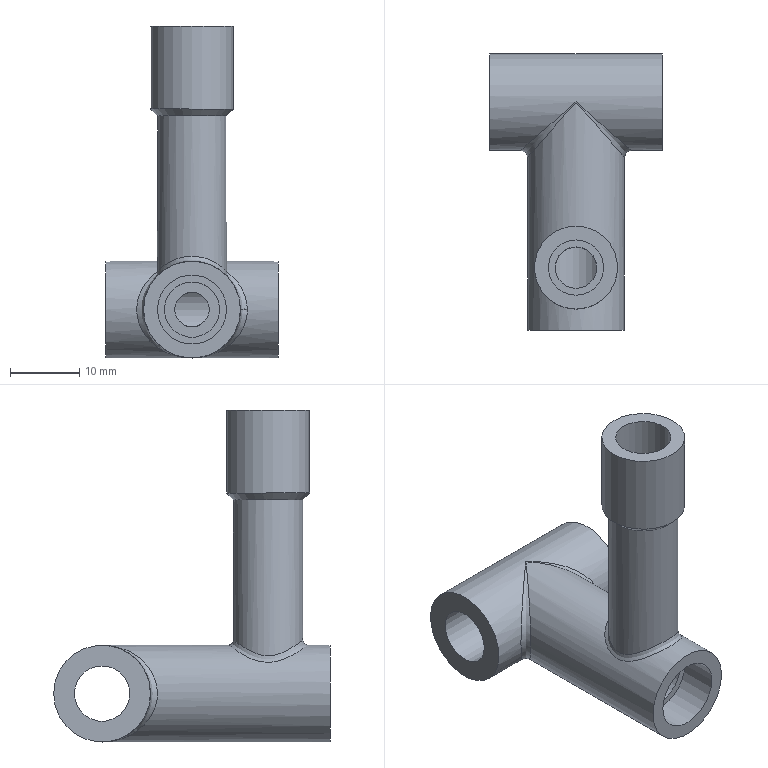Part | STEP file | 1-11.1 | 1 solid | 22 faces | box 25 x 40 x 48 mm | volume 7483 mm3 | cylinder 10 | plane 7 | spline 4 | cone 1 | commonest cylinder face diameters 8 x3 10 x2 14 x2 5 x1 6 x1 12 x1